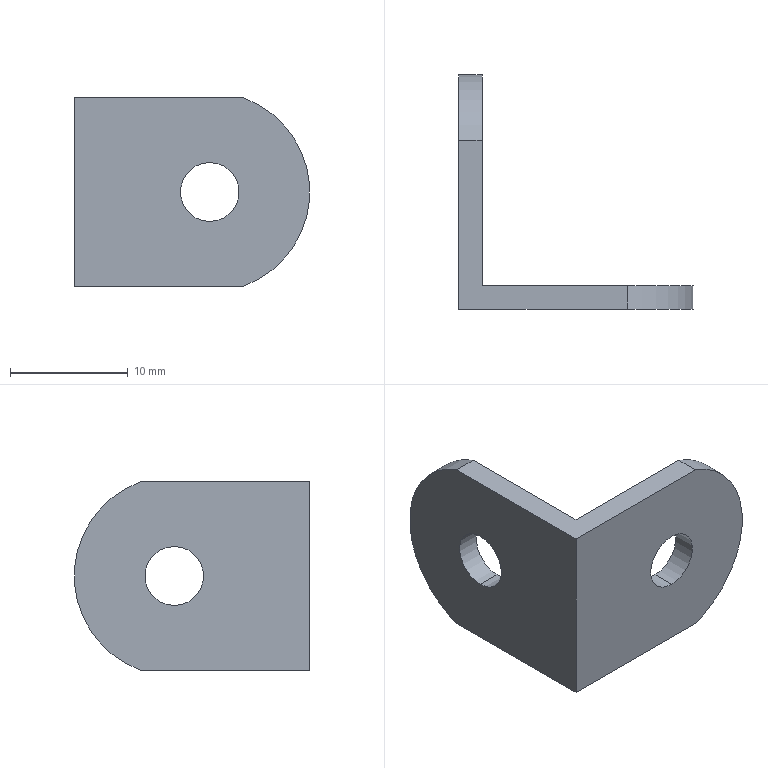Part | SolidWorks | features BaseBody 1 | 1 solid | 12 faces | box 20 x 20 x 16 mm | volume 1040 mm3 | cylinder 6 | plane 6 | commonest cylinder face diameters 5 x4 17 x2
STEP:
#1=CARTESIAN_POINT('',(0.,11.5,-2.5));
#2=VERTEX_POINT('',#1);
#3=CARTESIAN_POINT('',(0.,11.5,2.5));
#4=VERTEX_POINT('',#3);
#5=CARTESIAN_POINT('',(0.,11.5,0.));
#6=DIRECTION('',(-1.,0.,0.));
#7=DIRECTION('',(0.,0.,-1.));
#8=AXIS2_PLACEMENT_3D('',#5,#6,#7);
#9=CIRCLE('',#8,2.5);
#10=EDGE_CURVE('',#2,#4,#9,.T.);
#11=ORIENTED_EDGE('',*,*,#10,.T.);
#12=CARTESIAN_POINT('',(2.,11.5,2.5));
#13=VERTEX_POINT('',#12);
#14=CARTESIAN_POINT('',(-14.,11.5,2.5));
#15=DIRECTION('',(1.,0.,0.));
#16=VECTOR('',#15,1000.);
#17=LINE('',#14,#16);
#18=EDGE_CURVE('',#4,#13,#17,.T.);
#19=ORIENTED_EDGE('',*,*,#18,.T.);
#20=CARTESIAN_POINT('',(2.,11.5,-2.5));
#21=VERTEX_POINT('',#20);
#22=CARTESIAN_POINT('',(2.,11.5,0.));
#23=DIRECTION('',(-1.,0.,0.));
#24=DIRECTION('',(0.,0.,-1.));
#25=AXIS2_PLACEMENT_3D('',#22,#23,#24);
#26=CIRCLE('',#25,2.5);
#27=EDGE_CURVE('',#21,#13,#26,.T.);
#28=ORIENTED_EDGE('',*,*,#27,.F.);
#29=CARTESIAN_POINT('',(-14.,11.5,-2.5));
#30=DIRECTION('',(1.,0.,0.));
#31=VECTOR('',#30,1000.);
#32=LINE('',#29,#31);
#33=EDGE_CURVE('',#2,#21,#32,.T.);
#34=ORIENTED_EDGE('',*,*,#33,.F.);
#35=EDGE_LOOP('',(#11,#19,#28,#34));
#36=FACE_OUTER_BOUND('',#35,.T.);
#37=CARTESIAN_POINT('',(-14.,11.5,0.));
#38=DIRECTION('',(1.,0.,0.));
#39=DIRECTION('',(0.,0.,-1.));
#40=AXIS2_PLACEMENT_3D('',#37,#38,#39);
#41=CYLINDRICAL_SURFACE('',#40,2.5);
#42=ADVANCED_FACE('',(#36),#41,.F.);
#43=CARTESIAN_POINT('',(11.5,0.,2.5));
#44=VERTEX_POINT('',#43);
#45=CARTESIAN_POINT('',(11.5,0.,-2.5));
#46=VERTEX_POINT('',#45);
#47=CARTESIAN_POINT('',(11.5,0.,0.));
#48=DIRECTION('',(0.,-1.,0.));
#49=DIRECTION('',(0.,0.,1.));
#50=AXIS2_PLACEMENT_3D('',#47,#48,#49);
#51=CIRCLE('',#50,2.5);
#52=EDGE_CURVE('',#44,#46,#51,.T.);
#53=ORIENTED_EDGE('',*,*,#52,.T.);
#54=CARTESIAN_POINT('',(11.5,2.,-2.5));
#55=VERTEX_POINT('',#54);
#56=CARTESIAN_POINT('',(11.5,-14.,-2.5));
#57=DIRECTION('',(0.,1.,0.));
#58=VECTOR('',#57,1000.);
#59=LINE('',#56,#58);
#60=EDGE_CURVE('',#46,#55,#59,.T.);
#61=ORIENTED_EDGE('',*,*,#60,.T.);
#62=CARTESIAN_POINT('',(11.5,2.,2.5));
#63=VERTEX_POINT('',#62);
#64=CARTESIAN_POINT('',(11.5,2.,0.));
#65=DIRECTION('',(0.,1.,0.));
#66=DIRECTION('',(0.,0.,1.));
#67=AXIS2_PLACEMENT_3D('',#64,#65,#66);
#68=CIRCLE('',#67,2.5);
#69=EDGE_CURVE('',#55,#63,#68,.T.);
#70=ORIENTED_EDGE('',*,*,#69,.T.);
#71=CARTESIAN_POINT('',(11.5,-14.,2.5));
#72=DIRECTION('',(0.,1.,0.));
#73=VECTOR('',#72,1000.);
#74=LINE('',#71,#73);
#75=EDGE_CURVE('',#44,#63,#74,.T.);
#76=ORIENTED_EDGE('',*,*,#75,.F.);
#77=EDGE_LOOP('',(#53,#61,#70,#76));
#78=FACE_OUTER_BOUND('',#77,.T.);
#79=CARTESIAN_POINT('',(11.5,-14.,0.));
#80=DIRECTION('',(0.,1.,0.));
#81=DIRECTION('',(0.,0.,1.));
#82=AXIS2_PLACEMENT_3D('',#79,#80,#81);
#83=CYLINDRICAL_SURFACE('',#82,2.5);
#84=ADVANCED_FACE('',(#78),#83,.F.);
#85=CARTESIAN_POINT('',(0.,14.372,-8.));
#86=VERTEX_POINT('',#85);
#87=CARTESIAN_POINT('',(0.,14.372,8.));
#88=VERTEX_POINT('',#87);
#89=CARTESIAN_POINT('',(0.,11.5,0.));
#90=DIRECTION('',(1.,0.,0.));
#91=DIRECTION('',(0.,0.,-1.));
#92=AXIS2_PLACEMENT_3D('',#89,#90,#91);
#93=CIRCLE('',#92,8.5);
#94=EDGE_CURVE('',#86,#88,#93,.T.);
#95=ORIENTED_EDGE('',*,*,#94,.F.);
#96=CARTESIAN_POINT('',(0.,0.,-8.));
#97=VERTEX_POINT('',#96);
#98=CARTESIAN_POINT('',(0.,0.,-8.));
#99=DIRECTION('',(0.,1.,0.));
#100=VECTOR('',#99,1000.);
#101=LINE('',#98,#100);
#102=EDGE_CURVE('',#97,#86,#101,.T.);
#103=ORIENTED_EDGE('',*,*,#102,.F.);
#104=CARTESIAN_POINT('',(0.,0.,8.));
#105=VERTEX_POINT('',#104);
#106=CARTESIAN_POINT('',(0.,0.,8.));
#107=DIRECTION('',(0.,0.,-1.));
#108=VECTOR('',#107,1000.);
#109=LINE('',#106,#108);
#110=EDGE_CURVE('',#105,#97,#109,.T.);
#111=ORIENTED_EDGE('',*,*,#110,.F.);
#112=CARTESIAN_POINT('',(0.,0.,8.));
#113=DIRECTION('',(0.,-1.,0.));
#114=VECTOR('',#113,1000.);
#115=LINE('',#112,#114);
#116=EDGE_CURVE('',#88,#105,#115,.T.);
#117=ORIENTED_EDGE('',*,*,#116,.F.);
#118=EDGE_LOOP('',(#95,#103,#111,#117));
#119=FACE_OUTER_BOUND('',#118,.T.);
#120=ORIENTED_EDGE('',*,*,#10,.F.);
#121=CARTESIAN_POINT('',(0.,11.5,0.));
#122=DIRECTION('',(-1.,0.,0.));
#123=DIRECTION('',(0.,0.,-1.));
#124=AXIS2_PLACEMENT_3D('',#121,#122,#123);
#125=CIRCLE('',#124,2.5);
#126=EDGE_CURVE('',#4,#2,#125,.T.);
#127=ORIENTED_EDGE('',*,*,#126,.F.);
#128=EDGE_LOOP('',(#120,#127));
#129=FACE_BOUND('',#128,.T.);
#130=CARTESIAN_POINT('',(0.,0.,8.));
#131=DIRECTION('',(1.,0.,0.));
#132=DIRECTION('',(0.,0.,-1.));
#133=AXIS2_PLACEMENT_3D('',#130,#131,#132);
#134=PLANE('',#133);
#135=ADVANCED_FACE('',(#119,#129),#134,.F.);
#136=CARTESIAN_POINT('',(2.,2.,8.));
#137=VERTEX_POINT('',#136);
#138=CARTESIAN_POINT('',(14.372,2.,8.));
#139=VERTEX_POINT('',#138);
#140=CARTESIAN_POINT('',(0.,2.,8.));
#141=DIRECTION('',(1.,0.,0.));
#142=VECTOR('',#141,1000.);
#143=LINE('',#140,#142);
#144=EDGE_CURVE('',#137,#139,#143,.T.);
#145=ORIENTED_EDGE('',*,*,#144,.F.);
#146=CARTESIAN_POINT('',(2.,14.372,8.));
#147=VERTEX_POINT('',#146);
#148=CARTESIAN_POINT('',(2.,0.,8.));
#149=DIRECTION('',(0.,-1.,0.));
#150=VECTOR('',#149,1000.);
#151=LINE('',#148,#150);
#152=EDGE_CURVE('',#147,#137,#151,.T.);
#153=ORIENTED_EDGE('',*,*,#152,.F.);
#154=CARTESIAN_POINT('',(0.,14.372,8.));
#155=DIRECTION('',(1.,0.,0.));
#156=VECTOR('',#155,1000.);
#157=LINE('',#154,#156);
#158=EDGE_CURVE('',#88,#147,#157,.T.);
#159=ORIENTED_EDGE('',*,*,#158,.F.);
#160=ORIENTED_EDGE('',*,*,#116,.T.);
#161=CARTESIAN_POINT('',(14.372,0.,8.));
#162=VERTEX_POINT('',#161);
#163=CARTESIAN_POINT('',(0.,0.,8.));
#164=DIRECTION('',(-1.,0.,0.));
#165=VECTOR('',#164,1000.);
#166=LINE('',#163,#165);
#167=EDGE_CURVE('',#162,#105,#166,.T.);
#168=ORIENTED_EDGE('',*,*,#167,.F.);
#169=CARTESIAN_POINT('',(14.372,0.,8.));
#170=DIRECTION('',(0.,-1.,0.));
#171=VECTOR('',#170,1000.);
#172=LINE('',#169,#171);
#173=EDGE_CURVE('',#139,#162,#172,.T.);
#174=ORIENTED_EDGE('',*,*,#173,.F.);
#175=EDGE_LOOP('',(#145,#153,#159,#160,#168,#174));
#176=FACE_OUTER_BOUND('',#175,.T.);
#177=CARTESIAN_POINT('',(0.,0.,8.));
#178=DIRECTION('',(0.,0.,-1.));
#179=DIRECTION('',(-1.,0.,0.));
#180=AXIS2_PLACEMENT_3D('',#177,#178,#179);
#181=PLANE('',#180);
#182=ADVANCED_FACE('',(#176),#181,.F.);
#183=CARTESIAN_POINT('',(2.,14.372,-8.));
#184=VERTEX_POINT('',#183);
#185=CARTESIAN_POINT('',(2.,11.5,0.));
#186=DIRECTION('',(-1.,0.,0.));
#187=DIRECTION('',(0.,0.,-1.));
#188=AXIS2_PLACEMENT_3D('',#185,#186,#187);
#189=CIRCLE('',#188,8.5);
#190=EDGE_CURVE('',#147,#184,#189,.T.);
#191=ORIENTED_EDGE('',*,*,#190,.T.);
#192=CARTESIAN_POINT('',(-14.,14.372,-8.));
#193=DIRECTION('',(-1.,0.,0.));
#194=VECTOR('',#193,1000.);
#195=LINE('',#192,#194);
#196=EDGE_CURVE('',#184,#86,#195,.T.);
#197=ORIENTED_EDGE('',*,*,#196,.T.);
#198=ORIENTED_EDGE('',*,*,#94,.T.);
#199=ORIENTED_EDGE('',*,*,#158,.T.);
#200=EDGE_LOOP('',(#191,#197,#198,#199));
#201=FACE_OUTER_BOUND('',#200,.T.);
#202=CARTESIAN_POINT('',(-14.,11.5,0.));
#203=DIRECTION('',(1.,0.,0.));
#204=DIRECTION('',(0.,0.,-1.));
#205=AXIS2_PLACEMENT_3D('',#202,#203,#204);
#206=CYLINDRICAL_SURFACE('',#205,8.5);
#207=ADVANCED_FACE('',(#201),#206,.T.);
#208=ORIENTED_EDGE('',*,*,#196,.F.);
#209=CARTESIAN_POINT('',(2.,2.,-8.));
#210=VERTEX_POINT('',#209);
#211=CARTESIAN_POINT('',(2.,0.,-8.));
#212=DIRECTION('',(0.,-1.,0.));
#213=VECTOR('',#212,1000.);
#214=LINE('',#211,#213);
#215=EDGE_CURVE('',#184,#210,#214,.T.);
#216=ORIENTED_EDGE('',*,*,#215,.T.);
#217=CARTESIAN_POINT('',(14.372,2.,-8.));
#218=VERTEX_POINT('',#217);
#219=CARTESIAN_POINT('',(0.,2.,-8.));
#220=DIRECTION('',(1.,0.,0.));
#221=VECTOR('',#220,1000.);
#222=LINE('',#219,#221);
#223=EDGE_CURVE('',#210,#218,#222,.T.);
#224=ORIENTED_EDGE('',*,*,#223,.T.);
#225=CARTESIAN_POINT('',(14.372,0.,-8.));
#226=VERTEX_POINT('',#225);
#227=CARTESIAN_POINT('',(14.372,0.,-8.));
#228=DIRECTION('',(0.,-1.,0.));
#229=VECTOR('',#228,1000.);
#230=LINE('',#227,#229);
#231=EDGE_CURVE('',#218,#226,#230,.T.);
#232=ORIENTED_EDGE('',*,*,#231,.T.);
#233=CARTESIAN_POINT('',(0.,0.,-8.));
#234=DIRECTION('',(-1.,0.,0.));
#235=VECTOR('',#234,1000.);
#236=LINE('',#233,#235);
#237=EDGE_CURVE('',#226,#97,#236,.T.);
#238=ORIENTED_EDGE('',*,*,#237,.T.);
#239=ORIENTED_EDGE('',*,*,#102,.T.);
#240=EDGE_LOOP('',(#208,#216,#224,#232,#238,#239));
#241=FACE_OUTER_BOUND('',#240,.T.);
#242=CARTESIAN_POINT('',(0.,0.,-8.));
#243=DIRECTION('',(0.,0.,-1.));
#244=DIRECTION('',(-1.,0.,0.));
#245=AXIS2_PLACEMENT_3D('',#242,#243,#244);
#246=PLANE('',#245);
#247=ADVANCED_FACE('',(#241),#246,.T.);
#248=ORIENTED_EDGE('',*,*,#167,.T.);
#249=ORIENTED_EDGE('',*,*,#110,.T.);
#250=ORIENTED_EDGE('',*,*,#237,.F.);
#251=CARTESIAN_POINT('',(11.5,0.,0.));
#252=DIRECTION('',(0.,1.,0.));
#253=DIRECTION('',(0.,0.,1.));
#254=AXIS2_PLACEMENT_3D('',#251,#252,#253);
#255=CIRCLE('',#254,8.5);
#256=EDGE_CURVE('',#162,#226,#255,.T.);
#257=ORIENTED_EDGE('',*,*,#256,.F.);
#258=EDGE_LOOP('',(#248,#249,#250,#257));
#259=FACE_OUTER_BOUND('',#258,.T.);
#260=ORIENTED_EDGE('',*,*,#52,.F.);
#261=CARTESIAN_POINT('',(11.5,0.,0.));
#262=DIRECTION('',(0.,-1.,0.));
#263=DIRECTION('',(0.,0.,1.));
#264=AXIS2_PLACEMENT_3D('',#261,#262,#263);
#265=CIRCLE('',#264,2.5);
#266=EDGE_CURVE('',#46,#44,#265,.T.);
#267=ORIENTED_EDGE('',*,*,#266,.F.);
#268=EDGE_LOOP('',(#260,#267));
#269=FACE_BOUND('',#268,.T.);
#270=CARTESIAN_POINT('',(20.,0.,8.));
#271=DIRECTION('',(0.,1.,0.));
#272=DIRECTION('',(0.,0.,1.));
#273=AXIS2_PLACEMENT_3D('',#270,#271,#272);
#274=PLANE('',#273);
#275=ADVANCED_FACE('',(#259,#269),#274,.F.);
#276=ORIENTED_EDGE('',*,*,#18,.F.);
#277=ORIENTED_EDGE('',*,*,#126,.T.);
#278=ORIENTED_EDGE('',*,*,#33,.T.);
#279=CARTESIAN_POINT('',(2.,11.5,0.));
#280=DIRECTION('',(-1.,0.,0.));
#281=DIRECTION('',(0.,0.,-1.));
#282=AXIS2_PLACEMENT_3D('',#279,#280,#281);
#283=CIRCLE('',#282,2.5);
#284=EDGE_CURVE('',#13,#21,#283,.T.);
#285=ORIENTED_EDGE('',*,*,#284,.F.);
#286=EDGE_LOOP('',(#276,#277,#278,#285));
#287=FACE_OUTER_BOUND('',#286,.T.);
#288=CARTESIAN_POINT('',(-14.,11.5,0.));
#289=DIRECTION('',(1.,0.,0.));
#290=DIRECTION('',(0.,0.,-1.));
#291=AXIS2_PLACEMENT_3D('',#288,#289,#290);
#292=CYLINDRICAL_SURFACE('',#291,2.5);
#293=ADVANCED_FACE('',(#287),#292,.F.);
#294=CARTESIAN_POINT('',(11.5,2.,0.));
#295=DIRECTION('',(0.,-1.,0.));
#296=DIRECTION('',(0.,0.,1.));
#297=AXIS2_PLACEMENT_3D('',#294,#295,#296);
#298=CIRCLE('',#297,8.5);
#299=EDGE_CURVE('',#218,#139,#298,.T.);
#300=ORIENTED_EDGE('',*,*,#299,.T.);
#301=ORIENTED_EDGE('',*,*,#173,.T.);
#302=ORIENTED_EDGE('',*,*,#256,.T.);
#303=ORIENTED_EDGE('',*,*,#231,.F.);
#304=EDGE_LOOP('',(#300,#301,#302,#303));
#305=FACE_OUTER_BOUND('',#304,.T.);
#306=CARTESIAN_POINT('',(11.5,-14.,0.));
#307=DIRECTION('',(0.,1.,0.));
#308=DIRECTION('',(0.,0.,1.));
#309=AXIS2_PLACEMENT_3D('',#306,#307,#308);
#310=CYLINDRICAL_SURFACE('',#309,8.5);
#311=ADVANCED_FACE('',(#305),#310,.T.);
#312=ORIENTED_EDGE('',*,*,#299,.F.);
#313=ORIENTED_EDGE('',*,*,#223,.F.);
#314=CARTESIAN_POINT('',(2.,2.,8.));
#315=DIRECTION('',(0.,0.,-1.));
#316=VECTOR('',#315,1000.);
#317=LINE('',#314,#316);
#318=EDGE_CURVE('',#137,#210,#317,.T.);
#319=ORIENTED_EDGE('',*,*,#318,.F.);
#320=ORIENTED_EDGE('',*,*,#144,.T.);
#321=EDGE_LOOP('',(#312,#313,#319,#320));
#322=FACE_OUTER_BOUND('',#321,.T.);
#323=CARTESIAN_POINT('',(11.5,2.,0.));
#324=DIRECTION('',(0.,1.,0.));
#325=DIRECTION('',(0.,0.,1.));
#326=AXIS2_PLACEMENT_3D('',#323,#324,#325);
#327=CIRCLE('',#326,2.5);
#328=EDGE_CURVE('',#63,#55,#327,.T.);
#329=ORIENTED_EDGE('',*,*,#328,.F.);
#330=ORIENTED_EDGE('',*,*,#69,.F.);
#331=EDGE_LOOP('',(#329,#330));
#332=FACE_BOUND('',#331,.T.);
#333=CARTESIAN_POINT('',(2.,2.,8.));
#334=DIRECTION('',(0.,-1.,0.));
#335=DIRECTION('',(0.,0.,-1.));
#336=AXIS2_PLACEMENT_3D('',#333,#334,#335);
#337=PLANE('',#336);
#338=ADVANCED_FACE('',(#322,#332),#337,.F.);
#339=ORIENTED_EDGE('',*,*,#152,.T.);
#340=ORIENTED_EDGE('',*,*,#318,.T.);
#341=ORIENTED_EDGE('',*,*,#215,.F.);
#342=ORIENTED_EDGE('',*,*,#190,.F.);
#343=EDGE_LOOP('',(#339,#340,#341,#342));
#344=FACE_OUTER_BOUND('',#343,.T.);
#345=ORIENTED_EDGE('',*,*,#27,.T.);
#346=ORIENTED_EDGE('',*,*,#284,.T.);
#347=EDGE_LOOP('',(#345,#346));
#348=FACE_BOUND('',#347,.T.);
#349=CARTESIAN_POINT('',(2.,20.,8.));
#350=DIRECTION('',(-1.,0.,0.));
#351=DIRECTION('',(0.,0.,1.));
#352=AXIS2_PLACEMENT_3D('',#349,#350,#351);
#353=PLANE('',#352);
#354=ADVANCED_FACE('',(#344,#348),#353,.F.);
#355=ORIENTED_EDGE('',*,*,#60,.F.);
#356=ORIENTED_EDGE('',*,*,#266,.T.);
#357=ORIENTED_EDGE('',*,*,#75,.T.);
#358=ORIENTED_EDGE('',*,*,#328,.T.);
#359=EDGE_LOOP('',(#355,#356,#357,#358));
#360=FACE_OUTER_BOUND('',#359,.T.);
#361=CARTESIAN_POINT('',(11.5,-14.,0.));
#362=DIRECTION('',(0.,1.,0.));
#363=DIRECTION('',(0.,0.,1.));
#364=AXIS2_PLACEMENT_3D('',#361,#362,#363);
#365=CYLINDRICAL_SURFACE('',#364,2.5);
#366=ADVANCED_FACE('',(#360),#365,.F.);
#367=CLOSED_SHELL('',(#42,#84,#135,#182,#207,#247,#275,#293,#311,#338,#354,#366));
#368=MANIFOLD_SOLID_BREP('',#367);
#369=CARTESIAN_POINT('',(0.,0.,0.));
#370=DIRECTION('',(0.,0.,1.));
#371=DIRECTION('',(1.,0.,0.));
#372=AXIS2_PLACEMENT_3D('',#369,#370,#371);
#373=(LENGTH_UNIT()NAMED_UNIT(*)SI_UNIT(.MILLI.,.METRE.));
#374=UNCERTAINTY_MEASURE_WITH_UNIT(LENGTH_MEASURE(0.00001),#373,'','');
#375=(NAMED_UNIT(*)PLANE_ANGLE_UNIT()SI_UNIT($,.RADIAN.));
#376=(NAMED_UNIT(*)SI_UNIT($,.STERADIAN.)SOLID_ANGLE_UNIT());
#377=(GEOMETRIC_REPRESENTATION_CONTEXT(3)GLOBAL_UNCERTAINTY_ASSIGNED_CONTEXT((#374))GLOBAL_UNIT_ASSIGNED_CONTEXT((#373,#375,#376))REPRESENTATION_CONTEXT('',''));
#378=ADVANCED_BREP_SHAPE_REPRESENTATION('',(#368,#372),#377);